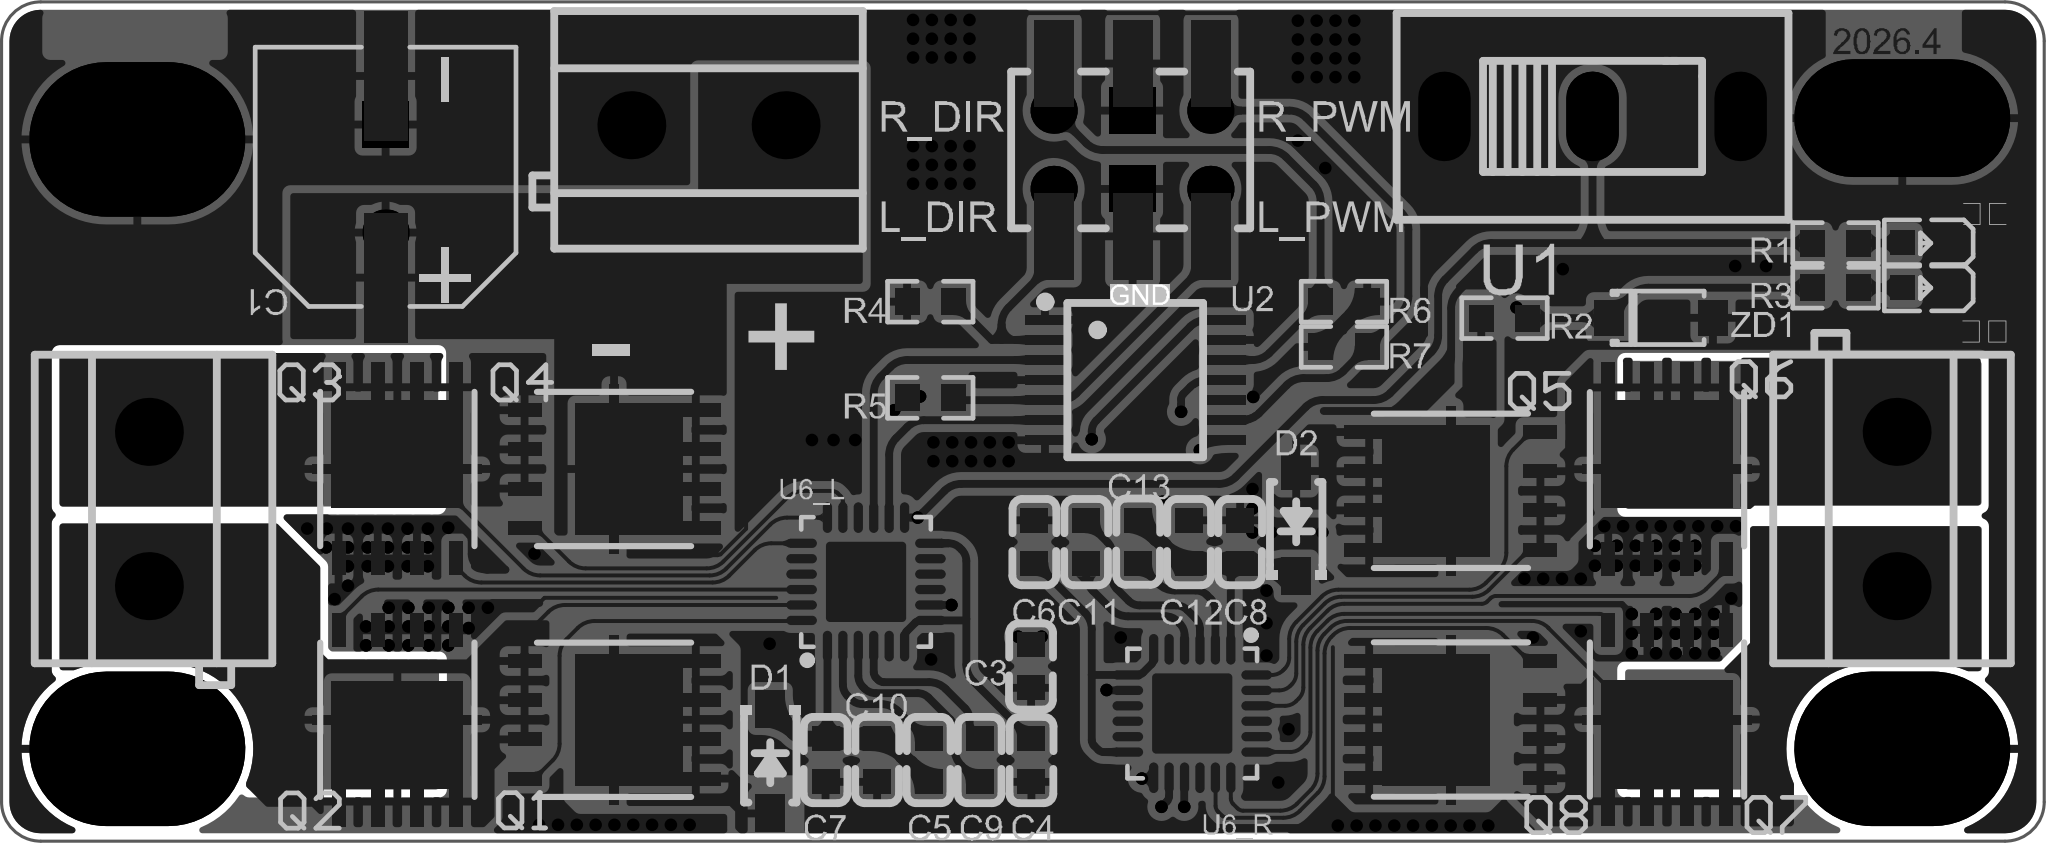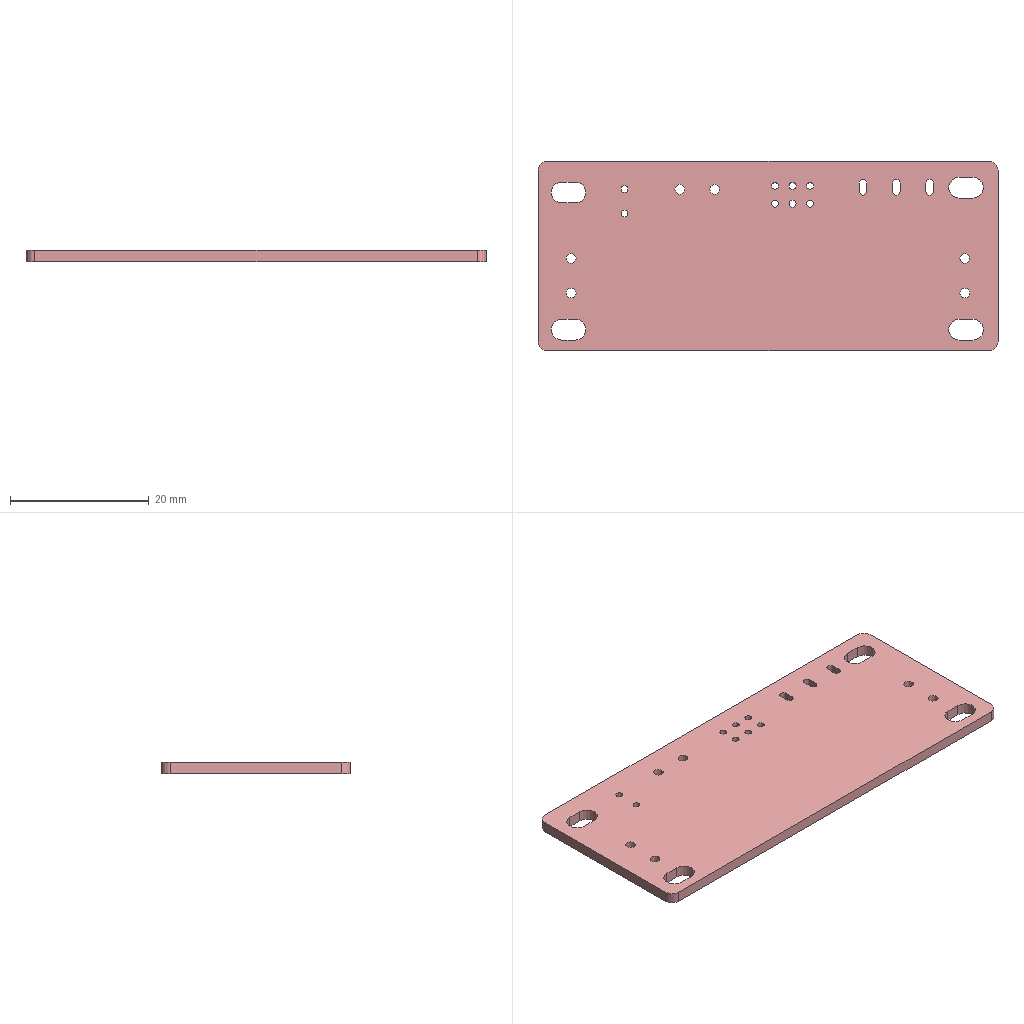Circuit board layout | Altium Designer | box 66.2 x 27.2 x 1.6 mm
Layer stack:
# Altium Designer layer stack of  (unit mm; dielectric type: 0 none, 1 core, 2 prepreg, 3 surface material)
index,name,kind,layer,copper_thickness_mm,dielectric_type,dielectric_thickness_mm,dielectric_material,dielectric_constant
0,Top Paste Mask Layer,other,,,,,,
1,Top Silkscreen Layer,other,,,,,,
2,Top Solder Mask Layer,dielectric,,,3,0.01,,3.3
3,Top Layer,copper,Top Layer,0.035,,,,
4,Dielectric1,dielectric,,,3,1.51,FR4,4.5
5,Bottom Layer,copper,Bottom Layer,0.035,,,,
6,Bottom Solder Mask Layer,dielectric,,,3,0.01,,3.3
7,Bottom Silkscreen Layer,other,,,,,,
8,Bottom Paste Mask Layer,other,,,,,,
# drill layer pairs: low layer,high layer
drill_pair,Top Layer,Bottom Layer
Part placement:
Designator,Comment,Layer,Footprint,Center-X(mm),Center-Y(mm),Rotation
C1,220uF,TopLayer,CAP-SMD_BD8.0-L8.3-W8.3-FD,88.646,97.826,90
C2,220uF,TopLayer,CAP-TH_BD8.0-P3.50-D0.6-FD,88.646,97.769,90
C3,1UF,TopLayer,C0603,109.566,81.964,90
C4,1UF,TopLayer,C0603,109.576,78.916,270
C5,1UF,TopLayer,C0603,106.248,78.932,90
C6,1UF,TopLayer,C0603,109.674,85.994,90
C7,10UF,TopLayer,C0603,102.904,78.916,270
C8,10UF,TopLayer,C0603,116.341,85.994,90
C9,100nF,TopLayer,C0603,107.902,78.932,90
C10,100nF,TopLayer,C0603,104.576,78.916,270
C11,100nF,TopLayer,C0603,111.348,85.979,270
C12,100nF,TopLayer,C0603,114.687,85.994,90
C13,1UF,TopLayer,C0603,113.033,85.994,270
D1,1N5819W,TopLayer,SOD-123_L2.7-W1.6-LS3.7-RD-1,101.112,78.894,270
D2,1N5819W,TopLayer,SOD-123_L2.7-W1.6-LS3.7-RD-1,118.158,86.59,90
H1,SMD,TopLayer,HDR-SMD_6P-P2.54-V-M-R2-C5-S7.4,112.856,98.696,0
K1,KF301-5.0-2P,TopLayer,CONN-TH_P5.00_KF301-5.0-2P,99.111,99.498,180
K2,KF301-5.0-2P,TopLayer,CONN-TH_P5.00_KF301-5.0-2P,137.617,87.06,90
K3,KF301-5.0-2P,TopLayer,CONN-TH_P5.00_KF301-5.0-2P,80.975,87.06,270
??,,TopLayer,LED_0603,138.608,94.236,180
M1,,TopLayer,M4螺丝,80.6,99.038,0
M2,,TopLayer,M4螺丝,137.8,99.727,0
M3,,TopLayer,M4螺丝,80.6,79.288,0
M4,,TopLayer,M4螺丝,137.8,79.288,0
R1,2.2K,TopLayer,R0603,135.636,95.679,180
R2,2.2K,TopLayer,R0603,124.908,93.246,180
R3,2.2K,TopLayer,R0603,135.636,94.231,180
R4,10K,TopLayer,R0603,106.299,93.778,180
R5,10K,TopLayer,R0603,106.299,90.662,180
R6,10K,TopLayer,R0603,119.705,93.778,180
R7,10K,TopLayer,R0603,119.705,92.313,0
U1,SS12D10G5,TopLayer,SW-TH_SHOU-HAN_SS12D10G4,127.762,99.783,0
U2,SN74HC125PWR,TopLayer,TSSOP-14_L5.0-W4.4-P0.65-LS6.5-BL,112.953,91.237,270
U6_L,DRV8701ERGET,TopLayer,VQFN-24_L4.0-W4.0-P0.50-BL-EP2.5,104.216,84.699,0
U6_R,DRV8701ERGET,TopLayer,VQFN-24_L4.0-W4.0-P0.50-BL-EP2.5,114.789,80.432,180
ZD1,BZT52C3V6,TopLayer,SOD-123_L2.8-W1.8-LS3.7-RD,129.972,93.256,0
??,,TopLayer,LED_0603,138.608,95.684,180
H2,,TopLayer,HDR-TH_6P-P2.54-V-R2-C3-S2.54_A2541WV-2X3P,112.837,98.701,0
Q1,TPH1R403NL,TopLayer,DFN5x6,95.925,80.228,270
Q2,TPH1R403NL,TopLayer,DFN5x6,89.027,80.353,180
Q3,TPH1R403NL,TopLayer,DFN5x6,89.027,88.231,0
Q4,TPH1R403NL,TopLayer,DFN5x6,95.925,88.356,270
Q5,TPH1R403NL,TopLayer,DFN5x6,123.297,87.649,90
Q6,TPH1R403NL,TopLayer,DFN5x6,130.175,88.224,0
Q7,TPH1R403NL,TopLayer,DFN5x6,130.175,80.363,180
Q8,TPH1R403NL,TopLayer,DFN5x6,123.297,80.238,90
Pad and via stacks:
# Altium Designer via and pad stacks of  (unit mm). Each distinct definition once, with the count of objects using it.
# via: kind,start_layer,end_layer,hole_mm,diameter_mm,mode(0 simple;1 top-mid-bottom;2 full stack),diameter_per_layer,count,example_net
# pad: kind,layer,hole_mm,hole_type(0 round;1 square;2 slot),plating,top_size,top_shape(1 round;2 rect;3 octagon;9 rounded rect),mid_size,bottom_size,mode,footprint,size_per_layer,count,example
pad,Top Layer,0,0,plated,4.2x1.4,2,4.2x1.4,4.2x1.4,0,CAP-SMD_BD8.0-L8.3-W8.3-FD,,2,C1.1
pad,Top Layer,0,0,plated,0.8x0.9,2,0.8x0.9,0.8x0.9,0,C0603,,22,C3.2
pad,Top Layer,0,0,plated,1.2x0.95,2,1.2x0.95,1.2x0.95,0,SOD-123_L2.7-W1.6-LS3.7-RD-1,,4,D1.2
pad,Top Layer,0,0,plated,1.27x2.8,2,1.27x2.8,1.27x2.8,0,HDR-SMD_6P-P2.54-V-M-R2-C5-S7.4,,6,H1.1
pad,Top Layer,0,0,plated,0.8001x0.8001,2,0.8001x0.8001,0.8001x0.8001,0,LED_0603,,4,\u7535\u6E90.1
pad,Top Layer,0,0,plated,0.8065x0.864,2,0.8065x0.864,0.8065x0.864,0,R0603,,14,R1.2
pad,Top Layer,0,0,plated,0.3048x1.27,2,0.3048x1.27,0.3048x1.27,0,TSSOP-14_L5.0-W4.4-P0.65-LS6.5-BL,,14,U2.1
pad,Top Layer,0,0,plated,2.6x2.6,9,2.6x2.6,2.6x2.6,0,VQFN-24_L4.0-W4.0-P0.50-BL-EP2.5,,2,U6_L.25
pad,Top Layer,0,0,plated,0.3x0.9906,9,0.3x0.9906,0.3x0.9906,0,VQFN-24_L4.0-W4.0-P0.50-BL-EP2.5,,48,U6_L.24
pad,Top Layer,0,0,plated,0.95x1.15,2,0.95x1.15,0.95x1.15,0,SOD-123_L2.8-W1.8-LS3.7-RD,,2,ZD1.2
pad,Top Layer,0,0,plated,4.25x3.5,2,4.25x3.5,4.25x3.5,0,DFN5x6,,8,Q1.1
pad,Top Layer,0,0,plated,0.45x1.6,2,0.45x1.6,0.45x1.6,0,DFN5x6,,32,Q1.1
pad,Top Layer,0,0,plated,0.45x1.1,2,0.45x1.1,0.45x1.1,0,DFN5x6,,32,Q1.3
pad,Top Layer,0,0,plated,5.5x0.3,2,5.5x0.3,5.5x0.3,0,DFN5x6,,8,Q1.1
pad,Multi-Layer,0.9906,0,plated,1.499x1.499,2,1.499x1.499,1.499x1.499,0,CAP-TH_BD8.0-P3.50-D0.6-FD,,1,C2.2
pad,Multi-Layer,0.9906,0,plated,1.499x1.499,1,1.499x1.499,1.499x1.499,0,CAP-TH_BD8.0-P3.50-D0.6-FD,,1,C2.1
pad,Multi-Layer,1.4,0,plated,2.2x2.2,1,2.2x2.2,2.2x2.2,0,CONN-TH_P5.00_KF301-5.0-2P,,6,K1.1
pad,Multi-Layer,3,2,plated,7x5,1,7x5,7x5,0,M4\u00C2\u00DD\u00CB\u00BF,,3,M1.1
pad,Multi-Layer,3,2,plated,7x3.81,1,7x3.81,7x3.81,0,M4\u00C2\u00DD\u00CB\u00BF,,1,M2.1
pad,Multi-Layer,1.1,2,plated,1.7x2.9,1,1.7x2.9,1.7x2.9,0,SW-TH_SHOU-HAN_SS12D10G4,,3,U1.1
pad,Multi-Layer,0.9906,0,plated,1.499x1.499,1,1.499x1.499,1.499x1.499,0,HDR-TH_6P-P2.54-V-R2-C3-S2.54_A2541WV-2X3P,,4,H2.1
pad,Multi-Layer,0.9906,0,plated,1.499x1.499,2,1.499x1.499,1.499x1.499,0,HDR-TH_6P-P2.54-V-R2-C3-S2.54_A2541WV-2X3P,,2,H2.3
via,Top Layer,Bottom Layer,0.3048,0.4064,0,,514,GND
Copper pours:
name,layer,net,type(0 solid;1 hatched;2 none)
Top Layer-VM,Top Layer,VM,0
Top Layer-VM 1,Top Layer,VM,0
Top Layer-L_A,Top Layer,L_A,0
Top Layer-R_A,Top Layer,R_A,0
Top Layer-R_B,Top Layer,R_B,0
Top Layer-VM 2,Top Layer,VM,0
Top Layer-VM 3,Top Layer,VM,0
Top Layer-VM 4,Top Layer,VM,0
Top Layer-GND,Top Layer,GND,0
Top Layer-L_B,Top Layer,L_B,0
Bottom Layer-VM,Bottom Layer,VM,0
Bottom Layer-VM 1,Bottom Layer,VM,0
Bottom Layer-VM 2,Bottom Layer,VM,0
Bottom Layer-VM 3,Bottom Layer,VM,0
Bottom Layer-GND,Bottom Layer,GND,0
Bottom Layer-R_A,Bottom Layer,R_A,0
Bottom Layer-R_B,Bottom Layer,R_B,0
Bottom Layer-L_B,Bottom Layer,L_B,0
Bottom Layer-L_A,Bottom Layer,L_A,0
Design rules, without the lines most boards share:
# Altium Designer design rules of  (exported by Altium Designer, unit mm)
# columns: name | kind | enabled | priority | scope1 | scope2 | descriptor | typed fields (field=value)
copperThickness2oz | 0 | disabled | 1 | All | All | Clearance Constraint (Gap=6mil) (Disabled)(All),(All) | gap=0.1524
Plane_innerPlane | 0 | disabled | 2 | All | All | Clearance Constraint (Gap=6mil) (Disabled)(All),(All) | gap=0.1524
Copper_copperRegion | 0 | disabled | 3 | All | All | Clearance Constraint (Gap=6mil) (Disabled)(All),(All) | gap=0.1524
Clearance | 0 | disabled | 4 | All | All | Clearance Constraint (Gap=6mil) (Disabled)(All),(All) | gap=0.1524
BoardOutlineClearance | 63 | disabled | 4 | All | All | Board Clearance Constraint (Gap=0mil) (Disabled)(All) |
Copper_18 | 0 | disabled | 5 | All | All | Clearance Constraint (Gap=6mil) (Disabled)(All),(All) | gap=0.1524
Copper_18_1 | 63 | disabled | 5 | All | All | Board Clearance Constraint (Gap=0mil) (Disabled)(All) |
Copper_18_copperThickness1oz | 0 | disabled | 6 | All | All | Clearance Constraint (Gap=6mil) (Disabled)(All),(All) | gap=0.1524
Copper_18_copperThickness1oz_1 | 63 | disabled | 6 | All | All | Board Clearance Constraint (Gap=0mil) (Disabled)(All) |
Copper_18_Copper_copperRegion | 0 | disabled | 7 | All | All | Clearance Constraint (Gap=6mil) (Disabled)(All),(All) | gap=0.1524
Copper_18_Copper_copperRegion_1 | 63 | disabled | 7 | All | All | Board Clearance Constraint (Gap=0mil) (Disabled)(All) |
Copper_copperRegion_Copper_18 | 0 | disabled | 8 | All | All | Clearance Constraint (Gap=6mil) (Disabled)(All),(All) | gap=0.1524
Copper_copperRegion_Copper_18_1 | 63 | disabled | 8 | All | All | Board Clearance Constraint (Gap=0mil) (Disabled)(All) |
Copper_copperRegion_Copper_copperRegion | 0 | disabled | 9 | All | All | Clearance Constraint (Gap=6mil) (Disabled)(All),(All) | gap=0.1524
Copper_copperRegion_Copper_copperRegion_1 | 63 | disabled | 9 | All | All | Board Clearance Constraint (Gap=0mil) (Disabled)(All) |
copperThickness1oz | 0 | enabled | 10 | All | All | Clearance Constraint (Gap=6mil) (All),(All) | gap=0.1524
copperThickness1oz_1 | 63 | enabled | 10 | All | All | Board Clearance Constraint (Gap=0mil) (All) |
otherClearance | 52 | enabled | 1 | All | All | Hole To Hole Clearance (Gap=11.8mil) (All),(All) | gap=0.2997
viaSize | 11 | enabled | 1 | All | All | Routing Via (MinHoleWidth=11.8mil) (MaxHoleWidth=248mil) (PreferredHoleWidth=12mil) (MinWidth=15.7mil) (MaxWidth=393.7mil) (PreferedWidth=24mil) (All) | via_min_hole=0.2997 via_max_hole=6.299 via_preferred_diameter=0.6096 via_preferred_hole=0.3048
PolygonConnect | 20 | disabled | 1 | All | All | Polygon Connect Rule(Direct Connect )(Conductor Width=10mil) (Relief Angle=90 Angle) (Entries=4) (Air Gap Width=10mil) (Disabled)(All),(All) | connect_style(0=relief,1=direct,2=none)=1 relief_conductor_width=0.254 relief_entries=4
18 | 20 | disabled | 2 | All | All | Polygon Connect Rule(Relief Connect )(Conductor Width=10mil) (Relief Angle=90 Angle) (Entries=4) (Air Gap Width=10mil) (Disabled)(All),(All) | connect_style(0=relief,1=direct,2=none)=0 relief_conductor_width=0.254 relief_entries=4
18_copperThickness1oz | 20 | disabled | 3 | All | All | Polygon Connect Rule(Relief Connect )(Conductor Width=10mil) (Relief Angle=90 Angle) (Entries=4) (Air Gap Width=10mil) (Disabled)(All),(All) | connect_style(0=relief,1=direct,2=none)=0 relief_conductor_width=0.254 relief_entries=4
18_Copper_copperRegion | 20 | disabled | 4 | All | All | Polygon Connect Rule(Relief Connect )(Conductor Width=10mil) (Relief Angle=90 Angle) (Entries=4) (Air Gap Width=10mil) (Disabled)(All),(All) | connect_style(0=relief,1=direct,2=none)=0 relief_conductor_width=0.254 relief_entries=4
copperRegion_Copper_18 | 20 | disabled | 5 | All | All | Polygon Connect Rule(Relief Connect )(Conductor Width=10mil) (Relief Angle=90 Angle) (Entries=4) (Air Gap Width=10mil) (Disabled)(All),(All) | connect_style(0=relief,1=direct,2=none)=0 relief_conductor_width=0.254 relief_entries=4
copperRegion_Copper_copperRegion | 20 | disabled | 6 | All | All | Polygon Connect Rule(Relief Connect )(Conductor Width=10mil) (Relief Angle=90 Angle) (Entries=4) (Air Gap Width=10mil) (Disabled)(All),(All) | connect_style(0=relief,1=direct,2=none)=0 relief_conductor_width=0.254 relief_entries=4
copperRegion | 20 | enabled | 7 | All | All | Polygon Connect Rule(Relief Connect )(Conductor Width=10mil) (Relief Angle=90 Angle) (Entries=4) (Air Gap Width=10mil) (All),(All) | connect_style(0=relief,1=direct,2=none)=0 relief_conductor_width=0.254 relief_entries=4